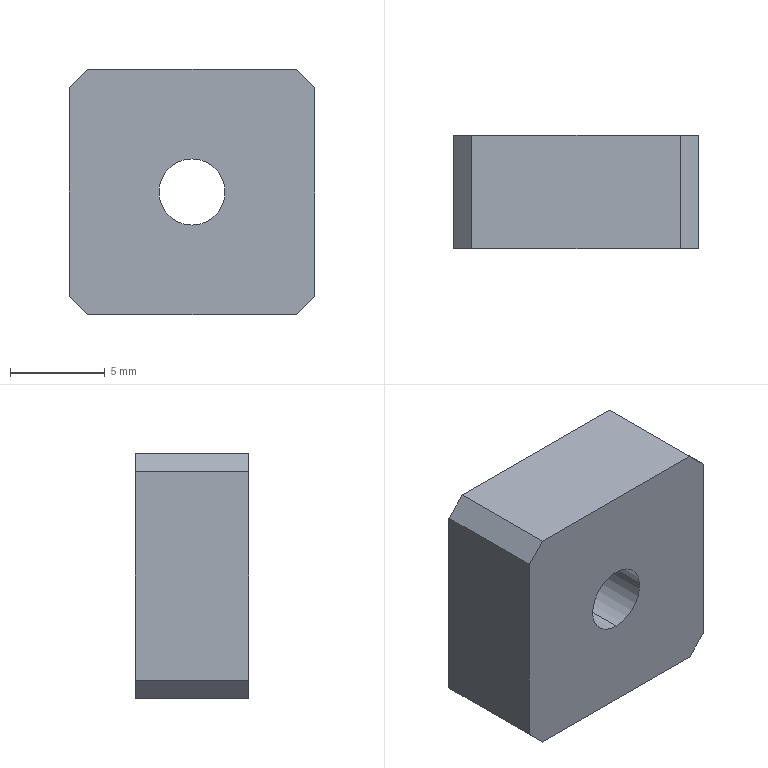Part | SolidWorks | features Chamfer 1, Extrusion 1, HoleWzd 1 | 1 solid | 12 faces | box 13 x 6 x 13 mm | volume 944.273 mm3 | plane 10 | cylinder 2 | commonest cylinder face diameters 3.5 x2
STEP:
#1=CARTESIAN_POINT('',(0.,0.,-1.75));
#2=VERTEX_POINT('',#1);
#3=CARTESIAN_POINT('',(0.,0.,1.75));
#4=VERTEX_POINT('',#3);
#5=CARTESIAN_POINT('',(0.,0.,0.));
#6=DIRECTION('',(0.,1.,0.));
#7=DIRECTION('',(0.,0.,1.));
#8=AXIS2_PLACEMENT_3D('',#5,#6,#7);
#9=CIRCLE('',#8,1.75);
#10=EDGE_CURVE('',#2,#4,#9,.T.);
#11=ORIENTED_EDGE('',*,*,#10,.F.);
#12=CARTESIAN_POINT('',(0.,6.,-1.75));
#13=VERTEX_POINT('',#12);
#14=CARTESIAN_POINT('',(0.,6.,-1.75));
#15=DIRECTION('',(0.,1.,0.));
#16=VECTOR('',#15,1000.);
#17=LINE('',#14,#16);
#18=EDGE_CURVE('',#2,#13,#17,.T.);
#19=ORIENTED_EDGE('',*,*,#18,.T.);
#20=CARTESIAN_POINT('',(0.,6.,1.75));
#21=VERTEX_POINT('',#20);
#22=CARTESIAN_POINT('',(0.,6.,0.));
#23=DIRECTION('',(0.,1.,0.));
#24=DIRECTION('',(0.,0.,1.));
#25=AXIS2_PLACEMENT_3D('',#22,#23,#24);
#26=CIRCLE('',#25,1.75);
#27=EDGE_CURVE('',#13,#21,#26,.T.);
#28=ORIENTED_EDGE('',*,*,#27,.T.);
#29=CARTESIAN_POINT('',(0.,6.,1.75));
#30=DIRECTION('',(0.,1.,0.));
#31=VECTOR('',#30,1000.);
#32=LINE('',#29,#31);
#33=EDGE_CURVE('',#4,#21,#32,.T.);
#34=ORIENTED_EDGE('',*,*,#33,.F.);
#35=EDGE_LOOP('',(#11,#19,#28,#34));
#36=FACE_OUTER_BOUND('',#35,.T.);
#37=CARTESIAN_POINT('',(0.,6.,0.));
#38=DIRECTION('',(0.,1.,0.));
#39=DIRECTION('',(0.,0.,1.));
#40=AXIS2_PLACEMENT_3D('',#37,#38,#39);
#41=CYLINDRICAL_SURFACE('',#40,1.75);
#42=ADVANCED_FACE('',(#36),#41,.F.);
#43=CARTESIAN_POINT('',(6.5,0.,5.5));
#44=VERTEX_POINT('',#43);
#45=CARTESIAN_POINT('',(6.5,0.,-5.5));
#46=VERTEX_POINT('',#45);
#47=CARTESIAN_POINT('',(6.5,0.,-6.5));
#48=DIRECTION('',(0.,0.,-1.));
#49=VECTOR('',#48,1000.);
#50=LINE('',#47,#49);
#51=EDGE_CURVE('',#44,#46,#50,.T.);
#52=ORIENTED_EDGE('',*,*,#51,.T.);
#53=CARTESIAN_POINT('',(6.5,6.,-5.5));
#54=VERTEX_POINT('',#53);
#55=CARTESIAN_POINT('',(6.5,6.,-5.5));
#56=DIRECTION('',(0.,1.,0.));
#57=VECTOR('',#56,1000.);
#58=LINE('',#55,#57);
#59=EDGE_CURVE('',#46,#54,#58,.T.);
#60=ORIENTED_EDGE('',*,*,#59,.T.);
#61=CARTESIAN_POINT('',(6.5,6.,5.5));
#62=VERTEX_POINT('',#61);
#63=CARTESIAN_POINT('',(6.5,6.,-6.5));
#64=DIRECTION('',(0.,0.,-1.));
#65=VECTOR('',#64,1000.);
#66=LINE('',#63,#65);
#67=EDGE_CURVE('',#62,#54,#66,.T.);
#68=ORIENTED_EDGE('',*,*,#67,.F.);
#69=CARTESIAN_POINT('',(6.5,6.,5.5));
#70=DIRECTION('',(0.,-1.,0.));
#71=VECTOR('',#70,1000.);
#72=LINE('',#69,#71);
#73=EDGE_CURVE('',#62,#44,#72,.T.);
#74=ORIENTED_EDGE('',*,*,#73,.T.);
#75=EDGE_LOOP('',(#52,#60,#68,#74));
#76=FACE_OUTER_BOUND('',#75,.T.);
#77=CARTESIAN_POINT('',(6.5,6.,-6.5));
#78=DIRECTION('',(-1.,0.,0.));
#79=DIRECTION('',(0.,0.,1.));
#80=AXIS2_PLACEMENT_3D('',#77,#78,#79);
#81=PLANE('',#80);
#82=ADVANCED_FACE('',(#76),#81,.F.);
#83=CARTESIAN_POINT('',(5.5,0.,-6.5));
#84=VERTEX_POINT('',#83);
#85=CARTESIAN_POINT('',(-5.5,0.,-6.5));
#86=VERTEX_POINT('',#85);
#87=CARTESIAN_POINT('',(-6.5,0.,-6.5));
#88=DIRECTION('',(-1.,0.,0.));
#89=VECTOR('',#88,1000.);
#90=LINE('',#87,#89);
#91=EDGE_CURVE('',#84,#86,#90,.T.);
#92=ORIENTED_EDGE('',*,*,#91,.T.);
#93=CARTESIAN_POINT('',(-5.5,6.,-6.5));
#94=VERTEX_POINT('',#93);
#95=CARTESIAN_POINT('',(-5.5,6.,-6.5));
#96=DIRECTION('',(0.,1.,0.));
#97=VECTOR('',#96,1000.);
#98=LINE('',#95,#97);
#99=EDGE_CURVE('',#86,#94,#98,.T.);
#100=ORIENTED_EDGE('',*,*,#99,.T.);
#101=CARTESIAN_POINT('',(5.5,6.,-6.5));
#102=VERTEX_POINT('',#101);
#103=CARTESIAN_POINT('',(-6.5,6.,-6.5));
#104=DIRECTION('',(-1.,0.,0.));
#105=VECTOR('',#104,1000.);
#106=LINE('',#103,#105);
#107=EDGE_CURVE('',#102,#94,#106,.T.);
#108=ORIENTED_EDGE('',*,*,#107,.F.);
#109=CARTESIAN_POINT('',(5.5,6.,-6.5));
#110=DIRECTION('',(0.,-1.,0.));
#111=VECTOR('',#110,1000.);
#112=LINE('',#109,#111);
#113=EDGE_CURVE('',#102,#84,#112,.T.);
#114=ORIENTED_EDGE('',*,*,#113,.T.);
#115=EDGE_LOOP('',(#92,#100,#108,#114));
#116=FACE_OUTER_BOUND('',#115,.T.);
#117=CARTESIAN_POINT('',(-6.5,6.,-6.5));
#118=DIRECTION('',(0.,0.,1.));
#119=DIRECTION('',(1.,0.,0.));
#120=AXIS2_PLACEMENT_3D('',#117,#118,#119);
#121=PLANE('',#120);
#122=ADVANCED_FACE('',(#116),#121,.F.);
#123=CARTESIAN_POINT('',(-6.5,6.,-5.5));
#124=VERTEX_POINT('',#123);
#125=CARTESIAN_POINT('',(-6.5,6.,5.5));
#126=VERTEX_POINT('',#125);
#127=CARTESIAN_POINT('',(-6.5,6.,-6.5));
#128=DIRECTION('',(0.,0.,1.));
#129=VECTOR('',#128,1000.);
#130=LINE('',#127,#129);
#131=EDGE_CURVE('',#124,#126,#130,.T.);
#132=ORIENTED_EDGE('',*,*,#131,.F.);
#133=CARTESIAN_POINT('',(-6.5,0.,-5.5));
#134=VERTEX_POINT('',#133);
#135=CARTESIAN_POINT('',(-6.5,6.,-5.5));
#136=DIRECTION('',(0.,-1.,0.));
#137=VECTOR('',#136,1000.);
#138=LINE('',#135,#137);
#139=EDGE_CURVE('',#124,#134,#138,.T.);
#140=ORIENTED_EDGE('',*,*,#139,.T.);
#141=CARTESIAN_POINT('',(-6.5,0.,5.5));
#142=VERTEX_POINT('',#141);
#143=CARTESIAN_POINT('',(-6.5,0.,-6.5));
#144=DIRECTION('',(0.,0.,1.));
#145=VECTOR('',#144,1000.);
#146=LINE('',#143,#145);
#147=EDGE_CURVE('',#134,#142,#146,.T.);
#148=ORIENTED_EDGE('',*,*,#147,.T.);
#149=CARTESIAN_POINT('',(-6.5,6.,5.5));
#150=DIRECTION('',(0.,1.,0.));
#151=VECTOR('',#150,1000.);
#152=LINE('',#149,#151);
#153=EDGE_CURVE('',#142,#126,#152,.T.);
#154=ORIENTED_EDGE('',*,*,#153,.T.);
#155=EDGE_LOOP('',(#132,#140,#148,#154));
#156=FACE_OUTER_BOUND('',#155,.T.);
#157=CARTESIAN_POINT('',(-6.5,6.,-6.5));
#158=DIRECTION('',(1.,0.,0.));
#159=DIRECTION('',(0.,0.,-1.));
#160=AXIS2_PLACEMENT_3D('',#157,#158,#159);
#161=PLANE('',#160);
#162=ADVANCED_FACE('',(#156),#161,.F.);
#163=CARTESIAN_POINT('',(-5.5,0.,6.5));
#164=VERTEX_POINT('',#163);
#165=CARTESIAN_POINT('',(5.5,0.,6.5));
#166=VERTEX_POINT('',#165);
#167=CARTESIAN_POINT('',(-6.5,0.,6.5));
#168=DIRECTION('',(1.,0.,0.));
#169=VECTOR('',#168,1000.);
#170=LINE('',#167,#169);
#171=EDGE_CURVE('',#164,#166,#170,.T.);
#172=ORIENTED_EDGE('',*,*,#171,.T.);
#173=CARTESIAN_POINT('',(5.5,6.,6.5));
#174=VERTEX_POINT('',#173);
#175=CARTESIAN_POINT('',(5.5,6.,6.5));
#176=DIRECTION('',(0.,1.,0.));
#177=VECTOR('',#176,1000.);
#178=LINE('',#175,#177);
#179=EDGE_CURVE('',#166,#174,#178,.T.);
#180=ORIENTED_EDGE('',*,*,#179,.T.);
#181=CARTESIAN_POINT('',(-5.5,6.,6.5));
#182=VERTEX_POINT('',#181);
#183=CARTESIAN_POINT('',(-6.5,6.,6.5));
#184=DIRECTION('',(1.,0.,0.));
#185=VECTOR('',#184,1000.);
#186=LINE('',#183,#185);
#187=EDGE_CURVE('',#182,#174,#186,.T.);
#188=ORIENTED_EDGE('',*,*,#187,.F.);
#189=CARTESIAN_POINT('',(-5.5,6.,6.5));
#190=DIRECTION('',(0.,-1.,0.));
#191=VECTOR('',#190,1000.);
#192=LINE('',#189,#191);
#193=EDGE_CURVE('',#182,#164,#192,.T.);
#194=ORIENTED_EDGE('',*,*,#193,.T.);
#195=EDGE_LOOP('',(#172,#180,#188,#194));
#196=FACE_OUTER_BOUND('',#195,.T.);
#197=CARTESIAN_POINT('',(-6.5,6.,6.5));
#198=DIRECTION('',(0.,0.,-1.));
#199=DIRECTION('',(-1.,0.,0.));
#200=AXIS2_PLACEMENT_3D('',#197,#198,#199);
#201=PLANE('',#200);
#202=ADVANCED_FACE('',(#196),#201,.F.);
#203=CARTESIAN_POINT('',(0.,6.,0.));
#204=DIRECTION('',(0.,1.,0.));
#205=DIRECTION('',(0.,0.,1.));
#206=AXIS2_PLACEMENT_3D('',#203,#204,#205);
#207=CIRCLE('',#206,1.75);
#208=EDGE_CURVE('',#21,#13,#207,.T.);
#209=ORIENTED_EDGE('',*,*,#208,.F.);
#210=ORIENTED_EDGE('',*,*,#27,.F.);
#211=EDGE_LOOP('',(#209,#210));
#212=FACE_BOUND('',#211,.T.);
#213=ORIENTED_EDGE('',*,*,#107,.T.);
#214=CARTESIAN_POINT('',(-6.,6.,-6.));
#215=DIRECTION('',(-0.7071,0.,0.7071));
#216=VECTOR('',#215,1000.);
#217=LINE('',#214,#216);
#218=EDGE_CURVE('',#94,#124,#217,.T.);
#219=ORIENTED_EDGE('',*,*,#218,.T.);
#220=ORIENTED_EDGE('',*,*,#131,.T.);
#221=CARTESIAN_POINT('',(-6.,6.,6.));
#222=DIRECTION('',(0.7071,0.,0.7071));
#223=VECTOR('',#222,1000.);
#224=LINE('',#221,#223);
#225=EDGE_CURVE('',#126,#182,#224,.T.);
#226=ORIENTED_EDGE('',*,*,#225,.T.);
#227=ORIENTED_EDGE('',*,*,#187,.T.);
#228=CARTESIAN_POINT('',(6.,6.,6.));
#229=DIRECTION('',(0.7071,0.,-0.7071));
#230=VECTOR('',#229,1000.);
#231=LINE('',#228,#230);
#232=EDGE_CURVE('',#174,#62,#231,.T.);
#233=ORIENTED_EDGE('',*,*,#232,.T.);
#234=ORIENTED_EDGE('',*,*,#67,.T.);
#235=CARTESIAN_POINT('',(6.,6.,-6.));
#236=DIRECTION('',(-0.7071,0.,-0.7071));
#237=VECTOR('',#236,1000.);
#238=LINE('',#235,#237);
#239=EDGE_CURVE('',#54,#102,#238,.T.);
#240=ORIENTED_EDGE('',*,*,#239,.T.);
#241=EDGE_LOOP('',(#213,#219,#220,#226,#227,#233,#234,#240));
#242=FACE_OUTER_BOUND('',#241,.T.);
#243=CARTESIAN_POINT('',(0.,6.,0.));
#244=DIRECTION('',(0.,1.,0.));
#245=DIRECTION('',(0.,0.,1.));
#246=AXIS2_PLACEMENT_3D('',#243,#244,#245);
#247=PLANE('',#246);
#248=ADVANCED_FACE('',(#212,#242),#247,.T.);
#249=CARTESIAN_POINT('',(0.,0.,0.));
#250=DIRECTION('',(0.,1.,0.));
#251=DIRECTION('',(0.,0.,1.));
#252=AXIS2_PLACEMENT_3D('',#249,#250,#251);
#253=CIRCLE('',#252,1.75);
#254=EDGE_CURVE('',#4,#2,#253,.T.);
#255=ORIENTED_EDGE('',*,*,#254,.T.);
#256=ORIENTED_EDGE('',*,*,#10,.T.);
#257=EDGE_LOOP('',(#255,#256));
#258=FACE_BOUND('',#257,.T.);
#259=ORIENTED_EDGE('',*,*,#147,.F.);
#260=CARTESIAN_POINT('',(-6.5,0.,-5.5));
#261=DIRECTION('',(0.7071,0.,-0.7071));
#262=VECTOR('',#261,1000.);
#263=LINE('',#260,#262);
#264=EDGE_CURVE('',#134,#86,#263,.T.);
#265=ORIENTED_EDGE('',*,*,#264,.T.);
#266=ORIENTED_EDGE('',*,*,#91,.F.);
#267=CARTESIAN_POINT('',(5.5,0.,-6.5));
#268=DIRECTION('',(0.7071,0.,0.7071));
#269=VECTOR('',#268,1000.);
#270=LINE('',#267,#269);
#271=EDGE_CURVE('',#84,#46,#270,.T.);
#272=ORIENTED_EDGE('',*,*,#271,.T.);
#273=ORIENTED_EDGE('',*,*,#51,.F.);
#274=CARTESIAN_POINT('',(6.5,0.,5.5));
#275=DIRECTION('',(-0.7071,0.,0.7071));
#276=VECTOR('',#275,1000.);
#277=LINE('',#274,#276);
#278=EDGE_CURVE('',#44,#166,#277,.T.);
#279=ORIENTED_EDGE('',*,*,#278,.T.);
#280=ORIENTED_EDGE('',*,*,#171,.F.);
#281=CARTESIAN_POINT('',(-5.5,0.,6.5));
#282=DIRECTION('',(-0.7071,0.,-0.7071));
#283=VECTOR('',#282,1000.);
#284=LINE('',#281,#283);
#285=EDGE_CURVE('',#164,#142,#284,.T.);
#286=ORIENTED_EDGE('',*,*,#285,.T.);
#287=EDGE_LOOP('',(#259,#265,#266,#272,#273,#279,#280,#286));
#288=FACE_OUTER_BOUND('',#287,.T.);
#289=CARTESIAN_POINT('',(0.,0.,0.));
#290=DIRECTION('',(0.,1.,0.));
#291=DIRECTION('',(0.,0.,1.));
#292=AXIS2_PLACEMENT_3D('',#289,#290,#291);
#293=PLANE('',#292);
#294=ADVANCED_FACE('',(#258,#288),#293,.F.);
#295=ORIENTED_EDGE('',*,*,#18,.F.);
#296=ORIENTED_EDGE('',*,*,#254,.F.);
#297=ORIENTED_EDGE('',*,*,#33,.T.);
#298=ORIENTED_EDGE('',*,*,#208,.T.);
#299=EDGE_LOOP('',(#295,#296,#297,#298));
#300=FACE_OUTER_BOUND('',#299,.T.);
#301=CARTESIAN_POINT('',(0.,6.,0.));
#302=DIRECTION('',(0.,1.,0.));
#303=DIRECTION('',(0.,0.,1.));
#304=AXIS2_PLACEMENT_3D('',#301,#302,#303);
#305=CYLINDRICAL_SURFACE('',#304,1.75);
#306=ADVANCED_FACE('',(#300),#305,.F.);
#307=ORIENTED_EDGE('',*,*,#218,.F.);
#308=ORIENTED_EDGE('',*,*,#99,.F.);
#309=ORIENTED_EDGE('',*,*,#264,.F.);
#310=ORIENTED_EDGE('',*,*,#139,.F.);
#311=EDGE_LOOP('',(#307,#308,#309,#310));
#312=FACE_OUTER_BOUND('',#311,.T.);
#313=CARTESIAN_POINT('',(-6.5,6.,-5.5));
#314=DIRECTION('',(0.7071,0.,0.7071));
#315=DIRECTION('',(0.,-1.,0.));
#316=AXIS2_PLACEMENT_3D('',#313,#314,#315);
#317=PLANE('',#316);
#318=ADVANCED_FACE('',(#312),#317,.F.);
#319=ORIENTED_EDGE('',*,*,#239,.F.);
#320=ORIENTED_EDGE('',*,*,#59,.F.);
#321=ORIENTED_EDGE('',*,*,#271,.F.);
#322=ORIENTED_EDGE('',*,*,#113,.F.);
#323=EDGE_LOOP('',(#319,#320,#321,#322));
#324=FACE_OUTER_BOUND('',#323,.T.);
#325=CARTESIAN_POINT('',(5.5,6.,-6.5));
#326=DIRECTION('',(-0.7071,0.,0.7071));
#327=DIRECTION('',(0.,-1.,0.));
#328=AXIS2_PLACEMENT_3D('',#325,#326,#327);
#329=PLANE('',#328);
#330=ADVANCED_FACE('',(#324),#329,.F.);
#331=ORIENTED_EDGE('',*,*,#232,.F.);
#332=ORIENTED_EDGE('',*,*,#179,.F.);
#333=ORIENTED_EDGE('',*,*,#278,.F.);
#334=ORIENTED_EDGE('',*,*,#73,.F.);
#335=EDGE_LOOP('',(#331,#332,#333,#334));
#336=FACE_OUTER_BOUND('',#335,.T.);
#337=CARTESIAN_POINT('',(6.5,6.,5.5));
#338=DIRECTION('',(-0.7071,0.,-0.7071));
#339=DIRECTION('',(0.,-1.,0.));
#340=AXIS2_PLACEMENT_3D('',#337,#338,#339);
#341=PLANE('',#340);
#342=ADVANCED_FACE('',(#336),#341,.F.);
#343=ORIENTED_EDGE('',*,*,#225,.F.);
#344=ORIENTED_EDGE('',*,*,#153,.F.);
#345=ORIENTED_EDGE('',*,*,#285,.F.);
#346=ORIENTED_EDGE('',*,*,#193,.F.);
#347=EDGE_LOOP('',(#343,#344,#345,#346));
#348=FACE_OUTER_BOUND('',#347,.T.);
#349=CARTESIAN_POINT('',(-5.5,6.,6.5));
#350=DIRECTION('',(0.7071,0.,-0.7071));
#351=DIRECTION('',(0.,-1.,0.));
#352=AXIS2_PLACEMENT_3D('',#349,#350,#351);
#353=PLANE('',#352);
#354=ADVANCED_FACE('',(#348),#353,.F.);
#355=CLOSED_SHELL('',(#42,#82,#122,#162,#202,#248,#294,#306,#318,#330,#342,#354));
#356=MANIFOLD_SOLID_BREP('',#355);
#357=CARTESIAN_POINT('',(0.,0.,0.));
#358=DIRECTION('',(0.,0.,1.));
#359=DIRECTION('',(1.,0.,0.));
#360=AXIS2_PLACEMENT_3D('',#357,#358,#359);
#361=(LENGTH_UNIT()NAMED_UNIT(*)SI_UNIT(.MILLI.,.METRE.));
#362=UNCERTAINTY_MEASURE_WITH_UNIT(LENGTH_MEASURE(0.00001),#361,'','');
#363=(NAMED_UNIT(*)PLANE_ANGLE_UNIT()SI_UNIT($,.RADIAN.));
#364=(NAMED_UNIT(*)SI_UNIT($,.STERADIAN.)SOLID_ANGLE_UNIT());
#365=(GEOMETRIC_REPRESENTATION_CONTEXT(3)GLOBAL_UNCERTAINTY_ASSIGNED_CONTEXT((#362))GLOBAL_UNIT_ASSIGNED_CONTEXT((#361,#363,#364))REPRESENTATION_CONTEXT('',''));
#366=ADVANCED_BREP_SHAPE_REPRESENTATION('',(#356,#360),#365);